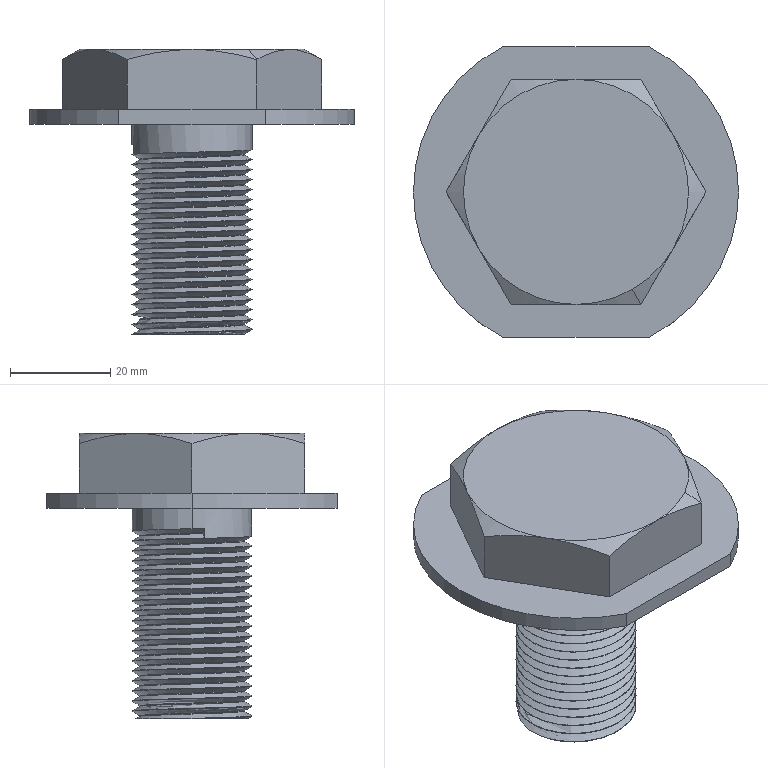Part | SolidWorks | features BaseBody 2 | 2 solids | 104 faces | box 65 x 58 x 57 mm | volume 47375 mm3 | cylinder 81 | plane 14 | cone 7 | spline 2 | commonest cylinder face diameters 21 x39 24 x39 65 x3